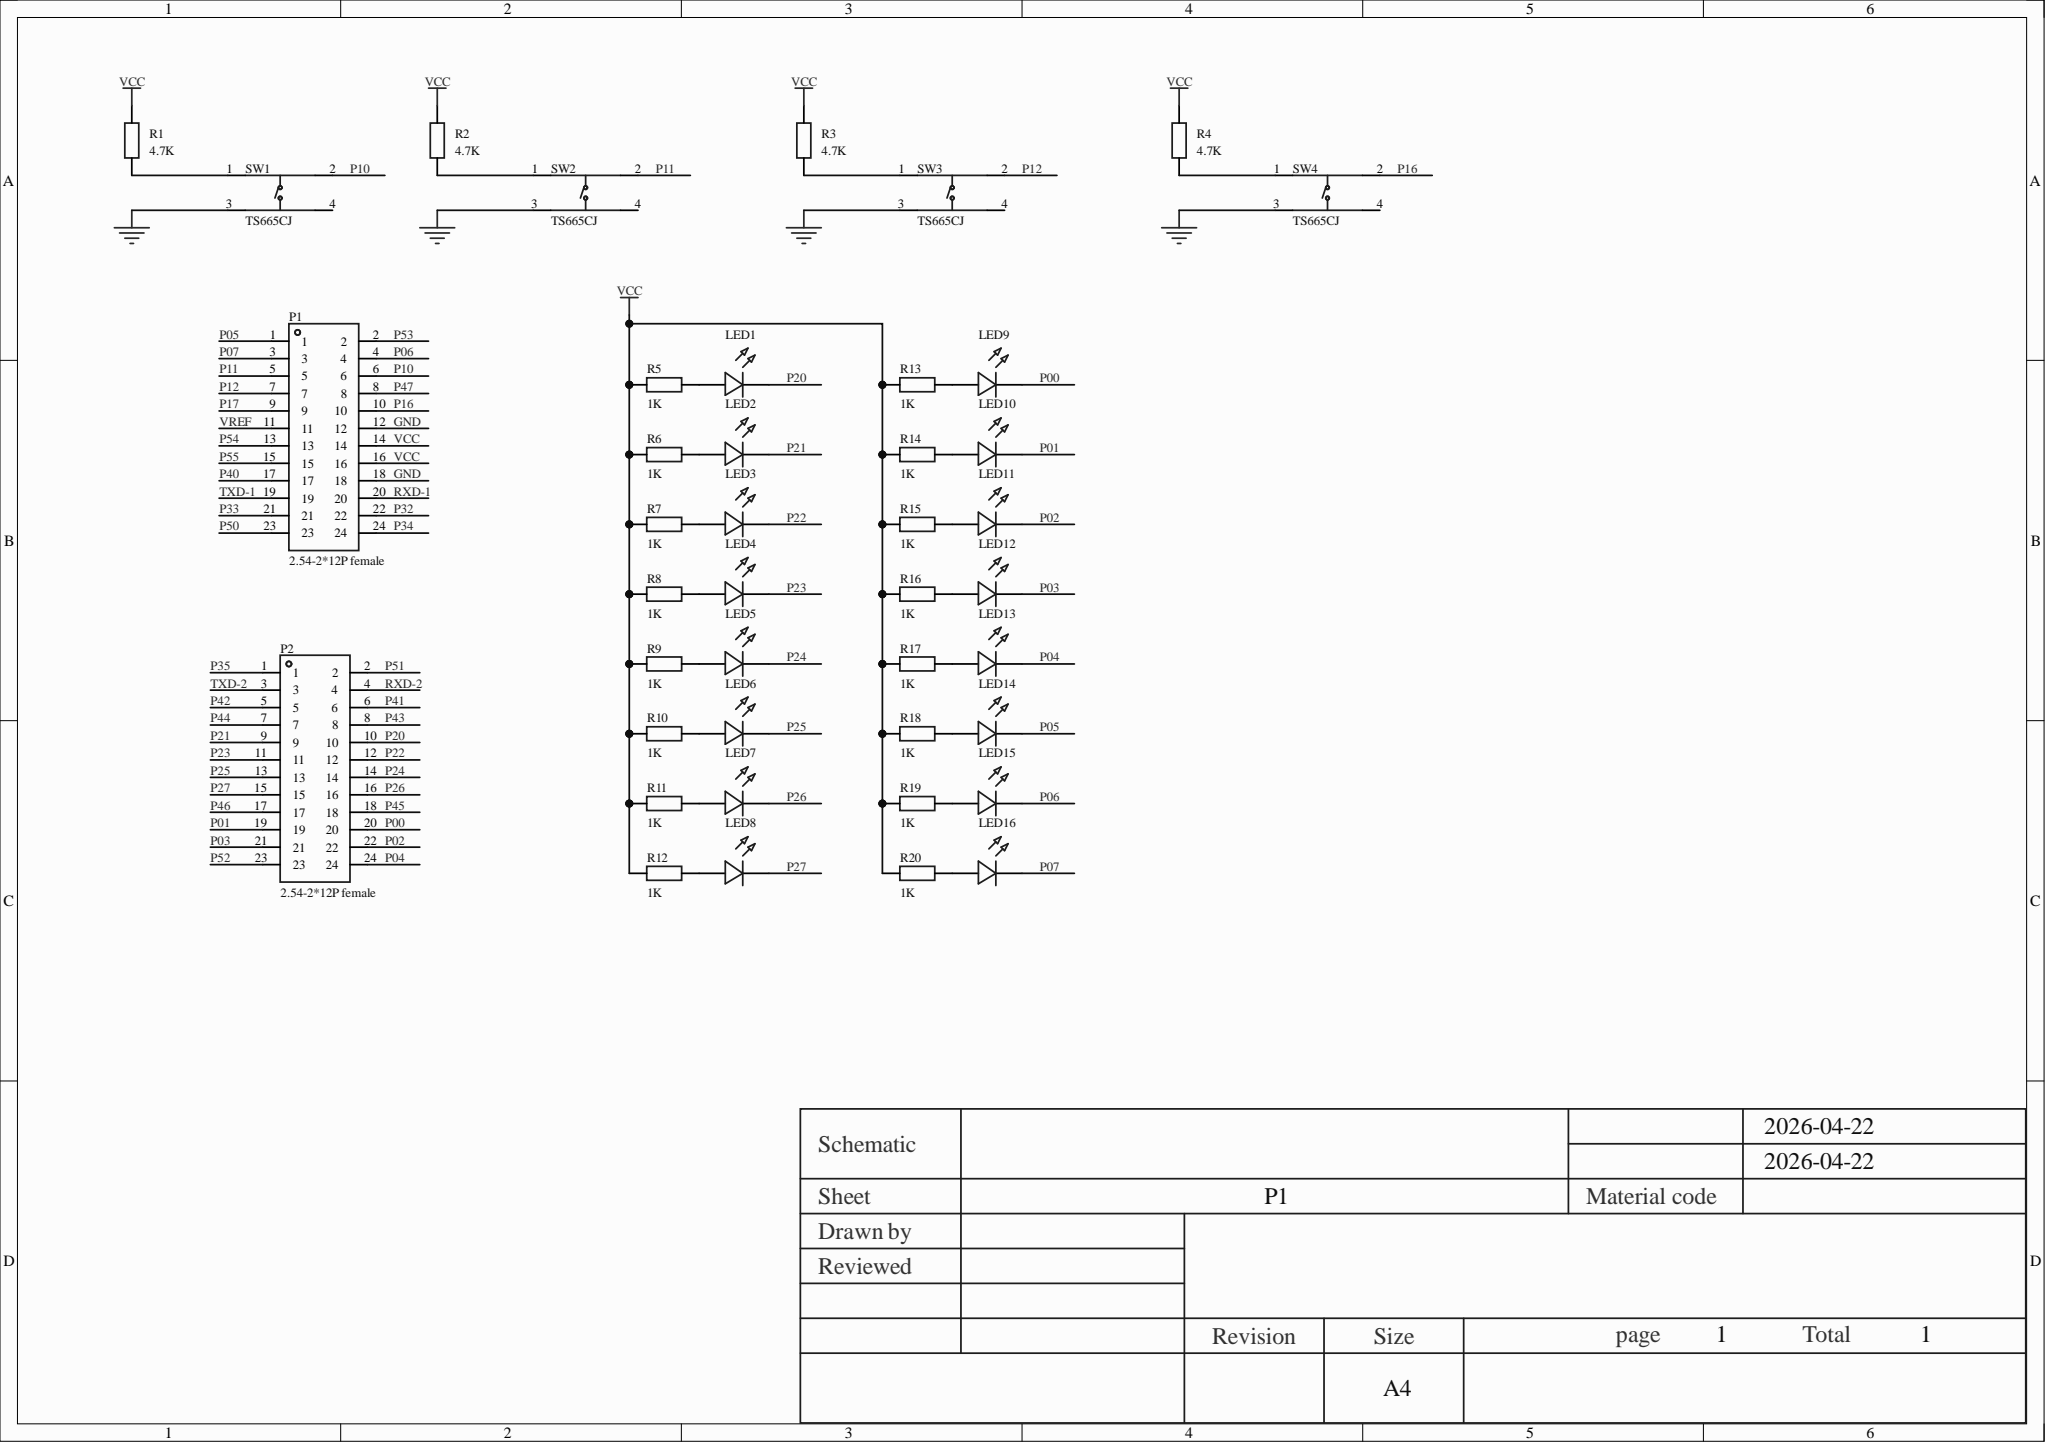Circuit board | Altium Designer | 42 parts | 42 nets
Bill of materials:
Comment,Description,Designator,Footprint,LibRef,Quantity
"","","LED1, LED2, LED3, LED4, LED5, LED6, LED7, LED8, LED9, LED10, LED11, LED12, LED13, LED14, LED15, LED16","LED-TH_L5.0-W5.0-P2.54_RED","LED_0603-G","16"
"2.54-2*12P female","Socket structure: 2x12P; pitch: 2.54mm; row spacing: 2.54mm; round/square hole: square hole; mounting: through-hole; rows: dual row; total positions: 24P; rated current: 3A; socket direction: top; plastic height: 2.5mm; contact material: brass; contact plating: -; operating temperature: -55℃~+105℃;","P1, P2","HDR-TH_24P-P2.54-V-F-R2-C12-S2.54","2.54-2*12P母","2"
"4.7K","","R1, R2, R3, R4","RES-TH_RES-TH_L6.5-W5.0-P2.50-D0.4-S2.00","Res_0603","4"
"1K","","R5, R6, R7, R8, R9, R10, R11, R12, R13, R14, R15, R16, R17, R18, R19, R20","RES-TH_RES-TH_L6.5-W5.0-P2.50-D0.4-S2.00","Res_0603","16"
"TS665CJ","Circuit: SPST; button shape: round; actuating force: 2.5N; mounting: through-hole; length: 6mm; width: 6mm; height: 5mm; bracket: none; contact current: 50mA; rated voltage: 12V; lamp: none; life: 5 ten-thousand cycles;","SW1, SW2, SW3, SW4","SW-TH_4P-L6.0-W6.0-P4.50-LS6.5","TS665CJ","4"
Netlist (Protel format):
[
LED1
LED-TH_L5.0-W5.0-P2.54_RED




]
[
LED2
LED-TH_L5.0-W5.0-P2.54_RED




]
[
LED3
LED-TH_L5.0-W5.0-P2.54_RED




]
[
LED4
LED-TH_L5.0-W5.0-P2.54_RED




]
[
LED5
LED-TH_L5.0-W5.0-P2.54_RED




]
[
LED6
LED-TH_L5.0-W5.0-P2.54_RED




]
[
LED7
LED-TH_L5.0-W5.0-P2.54_RED




]
[
LED8
LED-TH_L5.0-W5.0-P2.54_RED




]
[
LED9
LED-TH_L5.0-W5.0-P2.54_RED




]
[
LED10
LED-TH_L5.0-W5.0-P2.54_RED




]
[
LED11
LED-TH_L5.0-W5.0-P2.54_RED




]
[
LED12
LED-TH_L5.0-W5.0-P2.54_RED




]
[
LED13
LED-TH_L5.0-W5.0-P2.54_RED




]
[
LED14
LED-TH_L5.0-W5.0-P2.54_RED




]
[
LED15
LED-TH_L5.0-W5.0-P2.54_RED




]
[
LED16
LED-TH_L5.0-W5.0-P2.54_RED




]
[
P1
HDR-TH_24P-P2.54-V-F-R2-C12-S2.54
2.54-2*12P female



]
[
P2
HDR-TH_24P-P2.54-V-F-R2-C12-S2.54
2.54-2*12P female



]
[
R1
RES-TH_RES-TH_L6.5-W5.0-P2.50-D0.4-S2.00
4.7K



]
[
R2
RES-TH_RES-TH_L6.5-W5.0-P2.50-D0.4-S2.00
4.7K



]
[
R3
RES-TH_RES-TH_L6.5-W5.0-P2.50-D0.4-S2.00
4.7K



]
[
R4
RES-TH_RES-TH_L6.5-W5.0-P2.50-D0.4-S2.00
4.7K



]
[
R5
RES-TH_RES-TH_L6.5-W5.0-P2.50-D0.4-S2.00
1K



]
[
R6
RES-TH_RES-TH_L6.5-W5.0-P2.50-D0.4-S2.00
1K



]
[
R7
RES-TH_RES-TH_L6.5-W5.0-P2.50-D0.4-S2.00
1K



]
[
R8
RES-TH_RES-TH_L6.5-W5.0-P2.50-D0.4-S2.00
1K



]
[
R9
RES-TH_RES-TH_L6.5-W5.0-P2.50-D0.4-S2.00
1K



]
[
R10
RES-TH_RES-TH_L6.5-W5.0-P2.50-D0.4-S2.00
1K



]
[
R11
RES-TH_RES-TH_L6.5-W5.0-P2.50-D0.4-S2.00
1K



]
[
R12
RES-TH_RES-TH_L6.5-W5.0-P2.50-D0.4-S2.00
1K



]
[
R13
RES-TH_RES-TH_L6.5-W5.0-P2.50-D0.4-S2.00
1K



]
[
R14
RES-TH_RES-TH_L6.5-W5.0-P2.50-D0.4-S2.00
1K



]
[
R15
RES-TH_RES-TH_L6.5-W5.0-P2.50-D0.4-S2.00
1K



]
[
R16
RES-TH_RES-TH_L6.5-W5.0-P2.50-D0.4-S2.00
1K



]
[
R17
RES-TH_RES-TH_L6.5-W5.0-P2.50-D0.4-S2.00
1K



]
[
R18
RES-TH_RES-TH_L6.5-W5.0-P2.50-D0.4-S2.00
1K



]
[
R19
RES-TH_RES-TH_L6.5-W5.0-P2.50-D0.4-S2.00
1K



]
[
R20
RES-TH_RES-TH_L6.5-W5.0-P2.50-D0.4-S2.00
1K



]
[
SW1
SW-TH_4P-L6.0-W6.0-P4.50-LS6.5
TS665CJ



]
[
SW2
SW-TH_4P-L6.0-W6.0-P4.50-LS6.5
TS665CJ



]
[
SW3
SW-TH_4P-L6.0-W6.0-P4.50-LS6.5
TS665CJ



]
[
SW4
SW-TH_4P-L6.0-W6.0-P4.50-LS6.5
TS665CJ



]
(
VCC
P1-14
P1-16
R1-2
R2-2
R3-2
R4-2
R5-1
R6-1
R7-1
R8-1
R9-1
R10-1
R11-1
R12-1
R13-1
R14-1
R15-1
R16-1
R17-1
R18-1
R19-1
R20-1
)
(
P27
LED8-1
P2-15
)
(
P26
LED7-1
P2-16
)
(
P25
LED6-1
P2-13
)
(
P24
LED5-1
P2-14
)
(
P23
LED4-1
P2-11
)
(
P22
LED3-1
P2-12
)
(
P21
LED2-1
P2-9
)
(
P20
LED1-1
P2-10
)
(
P16
P1-10
SW4-2
)
(
P12
P1-7
SW3-2
)
(
P11
P1-5
SW2-2
)
(
P10
P1-6
SW1-2
)
(
P07
LED16-1
P1-3
)
(
P06
LED15-1
P1-4
)
(
P05
LED14-1
P1-1
)
(
P04
LED13-1
P2-24
)
(
P03
LED12-1
P2-21
)
(
P02
LED11-1
P2-22
)
(
P01
LED10-1
P2-19
)
(
P00
LED9-1
P2-20
)
(
NetR4_1
R4-1
SW4-1
)
(
NetR3_1
R3-1
SW3-1
)
(
NetR2_1
R2-1
SW2-1
)
(
NetR1_1
R1-1
SW1-1
)
(
NetLED16_2
LED16-2
R20-2
)
(
NetLED15_2
LED15-2
R19-2
)
(
NetLED14_2
LED14-2
R18-2
)
(
NetLED13_2
LED13-2
R17-2
)
(
NetLED12_2
LED12-2
R16-2
)
(
NetLED11_2
LED11-2
R15-2
)
(
NetLED10_2
LED10-2
R14-2
)
(
NetLED9_2
LED9-2
R13-2
)
(
NetLED8_2
LED8-2
R12-2
)
(
NetLED7_2
LED7-2
R11-2
)
(
NetLED6_2
LED6-2
R10-2
)
(
NetLED5_2
LED5-2
R9-2
)
(
NetLED4_2
LED4-2
R8-2
)
(
NetLED3_2
LED3-2
R7-2
)
(
NetLED2_2
LED2-2
R6-2
)
(
NetLED1_2
LED1-2
R5-2
)
(
GND
P1-12
P1-18
SW1-3
SW2-3
SW3-3
SW4-3
)